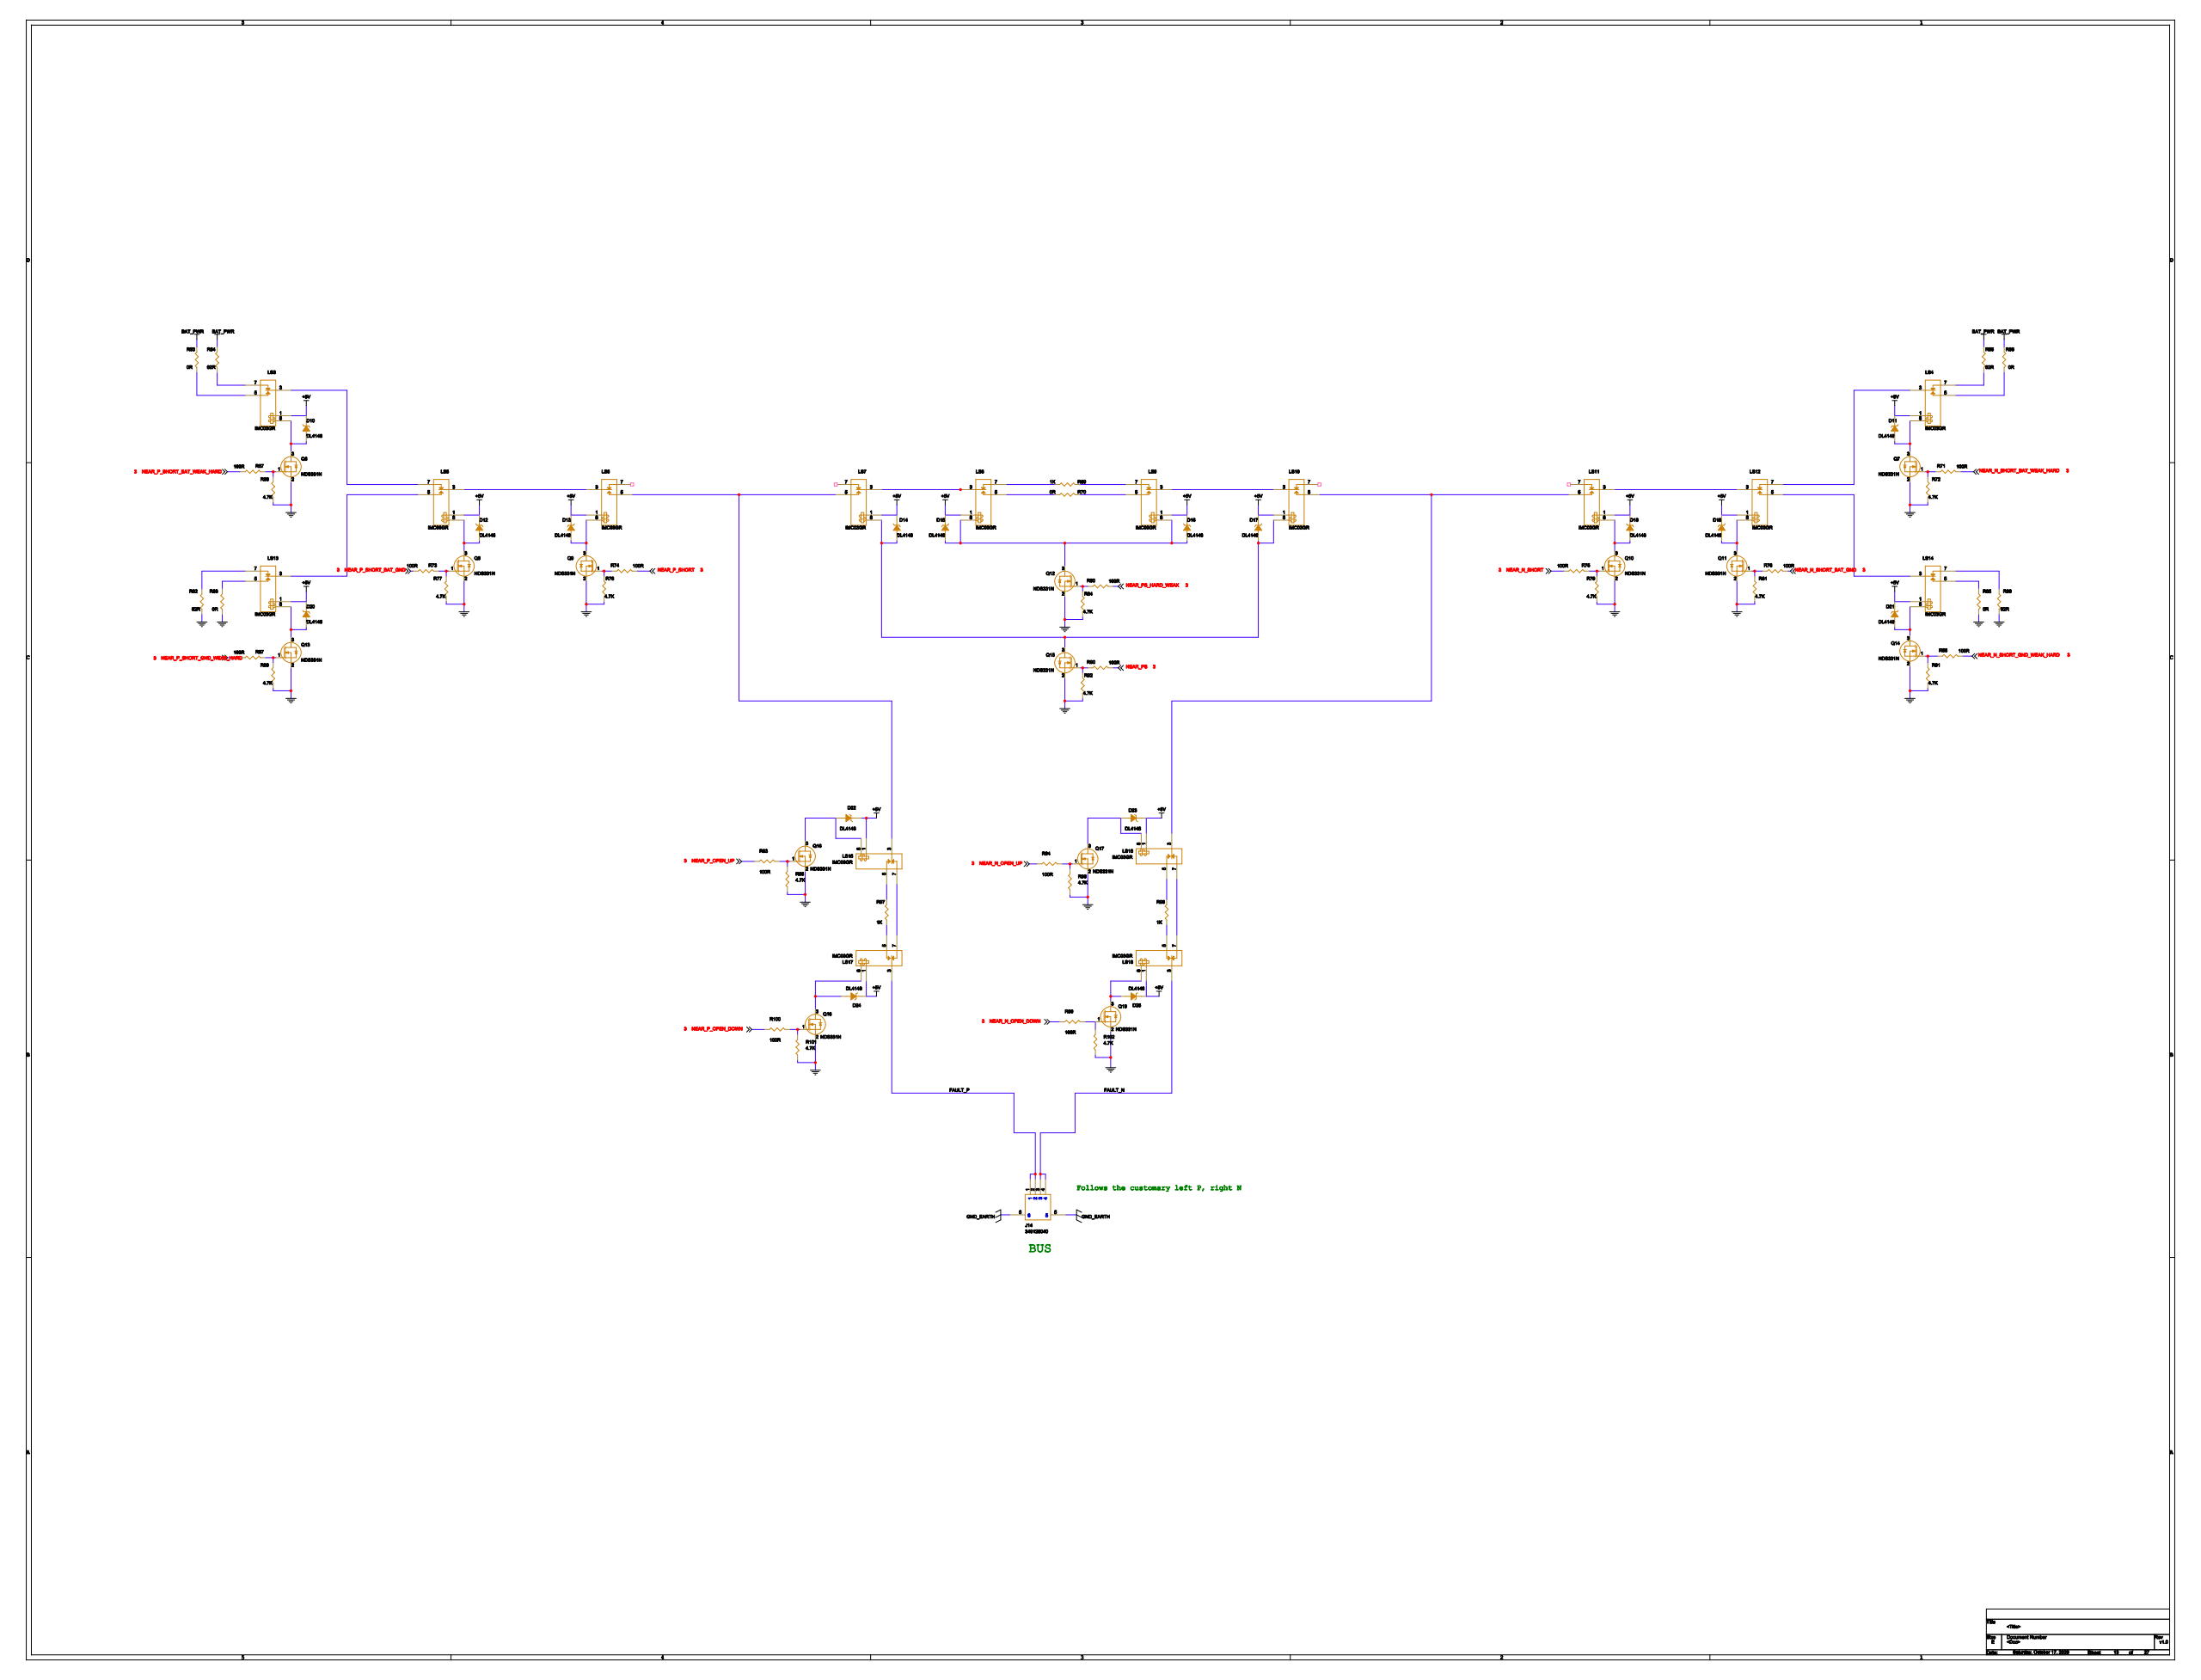Circuit board | Cadence Allegro | 477 parts | 327 nets | one sheet of the schematic
Parts on this sheet (reference | value | footprint):
D10 | DL4148 | MINIMELF
D11 | DL4148 | MINIMELF
D12 | DL4148 | MINIMELF
D13 | DL4148 | MINIMELF
D14 | DL4148 | MINIMELF
D15 | DL4148 | MINIMELF
D16 | DL4148 | MINIMELF
D17 | DL4148 | MINIMELF
D18 | DL4148 | MINIMELF
D19 | DL4148 | MINIMELF
D20 | DL4148 | MINIMELF
D21 | DL4148 | MINIMELF
D22 | DL4148 | MINIMELF
D23 | DL4148 | MINIMELF
D24 | DL4148 | MINIMELF
D25 | DL4148 | MINIMELF
J14 | 349128040 | 349128040
LS3 | IMC03GR | IMC03GR
LS4 | IMC03GR | IMC03GR
LS5 | IMC03GR | IMC03GR
LS6 | IMC03GR | IMC03GR
LS7 | IMC03GR | IMC03GR
LS8 | IMC03GR | IMC03GR
LS9 | IMC03GR | IMC03GR
LS10 | IMC03GR | IMC03GR
LS11 | IMC03GR | IMC03GR
LS12 | IMC03GR | IMC03GR
LS13 | IMC03GR | IMC03GR
LS14 | IMC03GR | IMC03GR
LS15 | IMC03GR | IMC03GR
LS16 | IMC03GR | IMC03GR
LS17 | IMC03GR | IMC03GR
LS18 | IMC03GR | IMC03GR
Q6 | NDS331N | SOT23-3
Q7 | NDS331N | SOT23-3
Q8 | NDS331N | SOT23-3
Q9 | NDS331N | SOT23-3
Q10 | NDS331N | SOT23-3
Q11 | NDS331N | SOT23-3
Q12 | NDS331N | SOT23-3
Q13 | NDS331N | SOT23-3
Q14 | NDS331N | SOT23-3
Q15 | NDS331N | SOT23-3
Q16 | NDS331N | SOT23-3
Q17 | NDS331N | SOT23-3
Q18 | NDS331N | SOT23-3
Q19 | NDS331N | SOT23-3
R63 | 0R | 0402
R64 | 62R | R0402
R65 | 62R | R0402
R66 | 0R | 0402
R67 | 100R | R0402
R68 | 4.7K | 0402
R69 | 1K | 0402
R70 | 0R | 0402
R71 | 100R | R0402
R72 | 4.7K | 0402
R73 | 100R | R0402
R74 | 100R | R0402
R75 | 100R | R0402
R76 | 100R | R0402
R77 | 4.7K | 0402
R78 | 4.7K | 0402
R79 | 4.7K | 0402
R80 | 100R | R0402
R81 | 4.7K | 0402
R82 | 62R | R0402
R83 | 0R | 0402
R84 | 4.7K | 0402
R85 | 0R | 0402
R86 | 62R | R0402
R87 | 100R | R0402
R88 | 100R | R0402
R89 | 4.7K | 0402
R90 | 100R | R0402
R91 | 4.7K | 0402
R92 | 4.7K | 0402
R93 | 100R | R0402
R94 | 100R | R0402
R95 | 4.7K | 0402
R96 | 4.7K | 0402
R97 | 1K | 0402
R98 | 1K | 0402
R99 | 100R | R0402
R100 | 100R | R0402
R101 | 4.7K | 0402
R102 | 4.7K | 0402
Nets of these parts (net: part-pin ...):
NEAR_P_OPEN_DOWN: R100-1
N20794: Q18-1 R100-2 R101-2
NEAR_P_SHORT_BAT_WEAK_HARD: R67-1
N03104: Q6-1 R67-2 R68-2
NEAR_N_SHORT_BAT_WEAK_HARD: R71-1
N11406: Q7-1 R71-2 R72-2
NEAR_P_SHORT_BAT_GND: R73-1
N04367: Q8-1 R73-2 R77-2
NEAR_P_SHORT: R74-1
N05175: Q9-1 R74-2 R78-2
NEAR_N_SHORT: R75-1
N11768: Q10-1 R75-2 R79-2
NEAR_N_SHORT_BAT_GND: R76-1
N11756: Q11-1 R76-2 R81-2
NEAR_PS_HARD_WEAK: R80-1
N07144: Q12-1 R80-2 R84-2
NEAR_P_SHORT_GND_WEAK_HARD: R87-1
N03834: Q13-1 R87-2 R89-2
NEAR_N_SHORT_GND_WEAK_HARD: R88-1
N12024: Q14-1 R88-2 R91-2
NEAR_PS: R90-1
N17934: Q15-1 R90-2 R92-2
NEAR_P_OPEN_UP: R93-1
N16457: Q16-1 R93-2 R95-2
NEAR_N_OPEN_UP: R94-1
N20231: Q17-1 R94-2 R96-2
NEAR_N_OPEN_DOWN: R99-1
N21286: Q19-1 R99-2 R102-2
GND: Q6-2 Q7-2 Q8-2 Q9-2 Q10-2 Q11-2 Q12-2 Q13-2 Q14-2 Q15-2 Q16-2 Q17-2 Q18-2 Q19-2 R68-1 R72-1 R77-1 R78-1 R79-1 R81-1 R82-1 R83-1 R84-1 R85-1 R86-1 R89-1 R91-1 R92-1 R95-1 R96-1 R101-1 R102-1
N06021: LS3-5 R63-1
BAT_PWR: R63-2 R64-2 R65-2 R66-2
N11254: LS4-5 R66-1
N07949: LS8-5 R70-1
N07945: LS9-5 R70-2
N06094: LS13-5 R83-2
N11790: LS14-5 R85-2
N05990: LS3-7 R64-1
N11258: LS4-7 R65-1
N03714: LS13-7 R82-2
N11744: LS14-7 R86-2
N07953: LS8-7 R69-1
N07941: LS9-7 R69-2
N16970: LS17-5 R97-1
N16966: LS15-5 R97-2
N20169: LS18-5 R98-1
N20133: LS16-5 R98-2
GND_EARTH: J14-5 J14-6
+5V: D10-2 D11-2 D12-2 D13-2 D14-2 D15-2 D16-2 D17-2 D18-2 D19-2 D20-2 D21-2 D22-2 D23-2 D24-2 D25-2 LS3-1 LS4-1 LS5-1 LS6-1 LS7-1 LS8-1 LS9-1 LS10-1 LS11-1 LS12-1 LS13-1 LS14-1 LS15-1 LS16-1 LS17-1 LS18-1
N11586: D18-1 LS11-8 Q10-3
N11550: D19-1 LS12-8 Q11-3
N07074: D15-1 D16-1 LS8-8 LS9-8 Q12-3
N03742: D20-1 LS13-8 Q13-3
N11910: D21-1 LS14-8 Q14-3
N08617: D14-1 D17-1 LS7-8 LS10-8 Q15-3
N15529: D22-1 LS15-8 Q16-3
N20083: D23-1 LS16-8 Q17-3
N20728: D24-1 LS17-8 Q18-3
N20297: D25-1 LS18-8 Q19-3
N01304: D10-1 LS3-8 Q6-3
N11316: D11-1 LS4-8 Q7-3
N04275: D12-1 LS5-8 Q8-3
N05083: D13-1 LS6-8 Q9-3
FAULT_P: J14-1 J14-2 LS17-3
FAULT_N: J14-3 J14-4 LS18-3
N07459: LS9-3 LS10-3
N12598: LS10-5 LS11-5 LS16-3
N11486: LS11-3 LS12-3
N11288: LS4-3 LS12-7
N11490: LS12-5 LS14-3
N01963: LS5-5 LS13-3
N09296: LS6-5 LS7-5 LS15-3
N16974: LS15-7 LS17-7
N20137: LS16-7 LS18-7
N01274: LS3-3 LS5-7
N04253: LS5-3 LS6-3
N09287: LS7-3 LS8-3